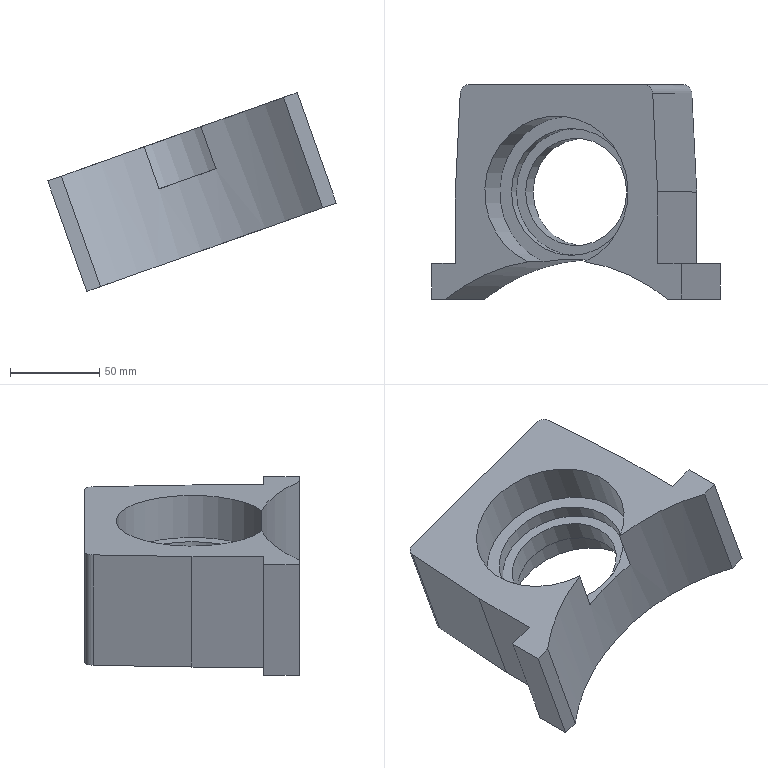Part | STEP file | SLIDE1-2_id582_x_t | 1 solid | 24 faces | box 161.375 x 120 x 111.146 mm | volume 535802 mm3 | plane 17 | cylinder 7 | commonest cylinder face diameters 10 x2 60 x1 71 x1 78 x1 85 x1 217 x1
STEP:
#1=CARTESIAN_POINT('',(-4.502,0.,-133.439));
#2=VERTEX_POINT('',#1);
#3=CARTESIAN_POINT('',(23.777,0.,-123.425));
#4=DIRECTION('',(-0.3338,0.,0.9426));
#5=DIRECTION('',(-0.9426,0.,-0.3338));
#6=AXIS2_PLACEMENT_3D('',#3,#4,#5);
#7=CIRCLE('',#6,30.);
#8=EDGE_CURVE('',#2,#2,#7,.T.);
#9=ORIENTED_EDGE('',*,*,#8,.F.);
#10=EDGE_LOOP('',(#9));
#11=FACE_BOUND('',#10,.T.);
#12=CARTESIAN_POINT('',(-8.675,0.,-121.656));
#13=VERTEX_POINT('',#12);
#14=CARTESIAN_POINT('',(19.605,0.,-111.642));
#15=DIRECTION('',(-0.3338,0.,0.9426));
#16=DIRECTION('',(-0.9426,0.,-0.3338));
#17=AXIS2_PLACEMENT_3D('',#14,#15,#16);
#18=CIRCLE('',#17,30.);
#19=EDGE_CURVE('',#13,#13,#18,.T.);
#20=ORIENTED_EDGE('',*,*,#19,.T.);
#21=EDGE_LOOP('',(#20));
#22=FACE_BOUND('',#21,.T.);
#23=CARTESIAN_POINT('',(23.777,0.,-123.425));
#24=DIRECTION('',(0.3338,0.,-0.9426));
#25=DIRECTION('',(-0.9426,0.,-0.3338));
#26=AXIS2_PLACEMENT_3D('',#23,#24,#25);
#27=CYLINDRICAL_SURFACE('',#26,30.);
#28=ADVANCED_FACE('',(#11,#22),#27,.F.);
#29=ORIENTED_EDGE('',*,*,#8,.T.);
#30=EDGE_LOOP('',(#29));
#31=FACE_BOUND('',#30,.T.);
#32=CARTESIAN_POINT('',(7.559,-35.,-129.168));
#33=VERTEX_POINT('',#32);
#34=CARTESIAN_POINT('',(39.995,-35.,-117.682));
#35=VERTEX_POINT('',#34);
#36=CARTESIAN_POINT('',(7.559,-35.,-129.168));
#37=DIRECTION('',(0.9426,0.,0.3338));
#38=VECTOR('',#37,1.);
#39=LINE('',#36,#38);
#40=EDGE_CURVE('',#33,#35,#39,.T.);
#41=ORIENTED_EDGE('',*,*,#40,.F.);
#42=CARTESIAN_POINT('',(23.777,0.,-123.425));
#43=DIRECTION('',(0.3338,0.,-0.9426));
#44=DIRECTION('',(-0.9426,0.,-0.3338));
#45=AXIS2_PLACEMENT_3D('',#42,#43,#44);
#46=CIRCLE('',#45,39.);
#47=EDGE_CURVE('',#33,#35,#46,.T.);
#48=ORIENTED_EDGE('',*,*,#47,.T.);
#49=EDGE_LOOP('',(#41,#48));
#50=FACE_BOUND('',#49,.T.);
#51=CARTESIAN_POINT('',(-32.781,60.,-143.453));
#52=DIRECTION('',(0.3338,0.,-0.9426));
#53=DIRECTION('',(-0.9426,0.,-0.3338));
#54=AXIS2_PLACEMENT_3D('',#51,#52,#53);
#55=PLANE('',#54);
#56=ADVANCED_FACE('',(#31,#50),#55,.T.);
#57=ORIENTED_EDGE('',*,*,#19,.F.);
#58=EDGE_LOOP('',(#57));
#59=FACE_BOUND('',#58,.T.);
#60=CARTESIAN_POINT('',(-13.859,0.,-123.492));
#61=VERTEX_POINT('',#60);
#62=CARTESIAN_POINT('',(19.605,0.,-111.642));
#63=DIRECTION('',(-0.3338,0.,0.9426));
#64=DIRECTION('',(-0.9426,0.,-0.3338));
#65=AXIS2_PLACEMENT_3D('',#62,#63,#64);
#66=CIRCLE('',#65,35.5);
#67=EDGE_CURVE('',#61,#61,#66,.T.);
#68=ORIENTED_EDGE('',*,*,#67,.T.);
#69=EDGE_LOOP('',(#68));
#70=FACE_BOUND('',#69,.T.);
#71=CARTESIAN_POINT('',(-36.954,60.,-131.67));
#72=DIRECTION('',(0.3338,0.,-0.9426));
#73=DIRECTION('',(-0.9426,0.,-0.3338));
#74=AXIS2_PLACEMENT_3D('',#71,#72,#73);
#75=PLANE('',#74);
#76=ADVANCED_FACE('',(#59,#70),#75,.F.);
#77=CARTESIAN_POINT('',(14.236,-35.,-148.021));
#78=VERTEX_POINT('',#77);
#79=CARTESIAN_POINT('',(14.236,-35.,-148.021));
#80=DIRECTION('',(-0.3338,0.,0.9426));
#81=VECTOR('',#80,1.);
#82=LINE('',#79,#81);
#83=EDGE_CURVE('',#78,#33,#82,.T.);
#84=ORIENTED_EDGE('',*,*,#83,.T.);
#85=ORIENTED_EDGE('',*,*,#40,.T.);
#86=CARTESIAN_POINT('',(46.671,-35.,-136.535));
#87=VERTEX_POINT('',#86);
#88=CARTESIAN_POINT('',(46.671,-35.,-136.535));
#89=DIRECTION('',(0.3338,0.,-0.9426));
#90=VECTOR('',#89,1.);
#91=LINE('',#88,#90);
#92=EDGE_CURVE('',#35,#87,#91,.T.);
#93=ORIENTED_EDGE('',*,*,#92,.T.);
#94=CARTESIAN_POINT('',(48.162,-35.,-136.007));
#95=DIRECTION('',(0.9426,0.,0.3338));
#96=VECTOR('',#95,1.);
#97=LINE('',#94,#96);
#98=EDGE_CURVE('',#78,#87,#97,.T.);
#99=ORIENTED_EDGE('',*,*,#98,.F.);
#100=EDGE_LOOP('',(#84,#85,#93,#99));
#101=FACE_OUTER_BOUND('',#100,.T.);
#102=CARTESIAN_POINT('',(7.559,-35.,-129.168));
#103=DIRECTION('',(0.,1.,0.));
#104=DIRECTION('',(0.,0.,1.));
#105=AXIS2_PLACEMENT_3D('',#102,#103,#104);
#106=PLANE('',#105);
#107=ADVANCED_FACE('',(#101),#106,.T.);
#108=ORIENTED_EDGE('',*,*,#47,.F.);
#109=ORIENTED_EDGE('',*,*,#83,.F.);
#110=CARTESIAN_POINT('',(30.453,0.,-142.278));
#111=DIRECTION('',(-0.3338,0.,0.9426));
#112=DIRECTION('',(-0.9426,0.,-0.3338));
#113=AXIS2_PLACEMENT_3D('',#110,#111,#112);
#114=CIRCLE('',#113,39.);
#115=EDGE_CURVE('',#87,#78,#114,.T.);
#116=ORIENTED_EDGE('',*,*,#115,.F.);
#117=ORIENTED_EDGE('',*,*,#92,.F.);
#118=EDGE_LOOP('',(#108,#109,#116,#117));
#119=FACE_OUTER_BOUND('',#118,.T.);
#120=CARTESIAN_POINT('',(30.453,0.,-142.278));
#121=DIRECTION('',(0.3338,0.,-0.9426));
#122=DIRECTION('',(-0.9426,0.,-0.3338));
#123=AXIS2_PLACEMENT_3D('',#120,#121,#122);
#124=CYLINDRICAL_SURFACE('',#123,39.);
#125=ADVANCED_FACE('',(#119),#124,.F.);
#126=ORIENTED_EDGE('',*,*,#67,.F.);
#127=EDGE_LOOP('',(#126));
#128=FACE_BOUND('',#127,.T.);
#129=CARTESIAN_POINT('',(-16.53,0.,-115.951));
#130=VERTEX_POINT('',#129);
#131=CARTESIAN_POINT('',(16.934,0.,-104.101));
#132=DIRECTION('',(-0.3338,0.,0.9426));
#133=DIRECTION('',(-0.9426,0.,-0.3338));
#134=AXIS2_PLACEMENT_3D('',#131,#132,#133);
#135=CIRCLE('',#134,35.5);
#136=EDGE_CURVE('',#130,#130,#135,.T.);
#137=ORIENTED_EDGE('',*,*,#136,.T.);
#138=EDGE_LOOP('',(#137));
#139=FACE_BOUND('',#138,.T.);
#140=CARTESIAN_POINT('',(19.605,0.,-111.642));
#141=DIRECTION('',(0.3338,0.,-0.9426));
#142=DIRECTION('',(-0.9426,0.,-0.3338));
#143=AXIS2_PLACEMENT_3D('',#140,#141,#142);
#144=CYLINDRICAL_SURFACE('',#143,35.5);
#145=ADVANCED_FACE('',(#128,#139),#144,.F.);
#146=CARTESIAN_POINT('',(57.711,60.,-63.14));
#147=VERTEX_POINT('',#146);
#148=CARTESIAN_POINT('',(62.418,55.262,-61.473));
#149=VERTEX_POINT('',#148);
#150=CARTESIAN_POINT('',(57.711,55.,-63.14));
#151=DIRECTION('',(0.3338,0.,-0.9426));
#152=DIRECTION('',(-0.9426,0.,-0.3338));
#153=AXIS2_PLACEMENT_3D('',#150,#151,#152);
#154=CIRCLE('',#153,5.);
#155=EDGE_CURVE('',#147,#149,#154,.T.);
#156=ORIENTED_EDGE('',*,*,#155,.T.);
#157=CARTESIAN_POINT('',(84.282,55.262,-123.216));
#158=VERTEX_POINT('',#157);
#159=CARTESIAN_POINT('',(62.418,55.262,-61.473));
#160=DIRECTION('',(0.3338,0.,-0.9426));
#161=VECTOR('',#160,1.);
#162=LINE('',#159,#161);
#163=EDGE_CURVE('',#149,#158,#162,.T.);
#164=ORIENTED_EDGE('',*,*,#163,.T.);
#165=CARTESIAN_POINT('',(79.575,60.,-124.883));
#166=VERTEX_POINT('',#165);
#167=CARTESIAN_POINT('',(79.575,55.,-124.883));
#168=DIRECTION('',(0.3338,0.,-0.9426));
#169=DIRECTION('',(-0.9426,0.,-0.3338));
#170=AXIS2_PLACEMENT_3D('',#167,#168,#169);
#171=CIRCLE('',#170,5.);
#172=EDGE_CURVE('',#166,#158,#171,.T.);
#173=ORIENTED_EDGE('',*,*,#172,.F.);
#174=CARTESIAN_POINT('',(57.711,60.,-63.14));
#175=DIRECTION('',(0.3338,0.,-0.9426));
#176=VECTOR('',#175,1.);
#177=LINE('',#174,#176);
#178=EDGE_CURVE('',#147,#166,#177,.T.);
#179=ORIENTED_EDGE('',*,*,#178,.F.);
#180=EDGE_LOOP('',(#156,#164,#173,#179));
#181=FACE_OUTER_BOUND('',#180,.T.);
#182=CARTESIAN_POINT('',(57.595,55.,-62.813));
#183=DIRECTION('',(0.3338,0.,-0.9426));
#184=DIRECTION('',(-0.9426,0.,-0.3338));
#185=AXIS2_PLACEMENT_3D('',#182,#183,#184);
#186=CYLINDRICAL_SURFACE('',#185,5.);
#187=ADVANCED_FACE('',(#181),#186,.T.);
#188=CARTESIAN_POINT('',(87.012,0.,-122.249));
#189=VERTEX_POINT('',#188);
#190=CARTESIAN_POINT('',(65.148,0.,-60.506));
#191=VERTEX_POINT('',#190);
#192=CARTESIAN_POINT('',(65.148,0.,-60.506));
#193=DIRECTION('',(-0.3338,0.,0.9426));
#194=VECTOR('',#193,1.);
#195=LINE('',#192,#194);
#196=EDGE_CURVE('',#189,#191,#195,.T.);
#197=ORIENTED_EDGE('',*,*,#196,.F.);
#198=CARTESIAN_POINT('',(84.282,55.262,-123.216));
#199=DIRECTION('',(0.04933,-0.9986,0.01747));
#200=VECTOR('',#199,1.);
#201=LINE('',#198,#200);
#202=EDGE_CURVE('',#158,#189,#201,.T.);
#203=ORIENTED_EDGE('',*,*,#202,.F.);
#204=ORIENTED_EDGE('',*,*,#163,.F.);
#205=CARTESIAN_POINT('',(62.418,55.262,-61.473));
#206=DIRECTION('',(0.04933,-0.9986,0.01747));
#207=VECTOR('',#206,1.);
#208=LINE('',#205,#207);
#209=EDGE_CURVE('',#149,#191,#208,.T.);
#210=ORIENTED_EDGE('',*,*,#209,.T.);
#211=EDGE_LOOP('',(#197,#203,#204,#210));
#212=FACE_OUTER_BOUND('',#211,.T.);
#213=CARTESIAN_POINT('',(62.183,60.,-61.556));
#214=DIRECTION('',(-0.9413,-0.05234,-0.3333));
#215=DIRECTION('',(-0.3338,0.,0.9426));
#216=AXIS2_PLACEMENT_3D('',#213,#214,#215);
#217=PLANE('',#216);
#218=ADVANCED_FACE('',(#212),#217,.F.);
#219=CARTESIAN_POINT('',(87.012,-40.,-122.249));
#220=VERTEX_POINT('',#219);
#221=CARTESIAN_POINT('',(87.012,60.,-122.249));
#222=DIRECTION('',(0.,-1.,0.));
#223=VECTOR('',#222,1.);
#224=LINE('',#221,#223);
#225=EDGE_CURVE('',#189,#220,#224,.T.);
#226=ORIENTED_EDGE('',*,*,#225,.F.);
#227=ORIENTED_EDGE('',*,*,#196,.T.);
#228=CARTESIAN_POINT('',(65.148,-40.,-60.506));
#229=VERTEX_POINT('',#228);
#230=CARTESIAN_POINT('',(65.148,60.,-60.506));
#231=DIRECTION('',(0.,-1.,0.));
#232=VECTOR('',#231,1.);
#233=LINE('',#230,#232);
#234=EDGE_CURVE('',#191,#229,#233,.T.);
#235=ORIENTED_EDGE('',*,*,#234,.T.);
#236=CARTESIAN_POINT('',(87.012,-40.,-122.249));
#237=DIRECTION('',(-0.3338,0.,0.9426));
#238=VECTOR('',#237,1.);
#239=LINE('',#236,#238);
#240=EDGE_CURVE('',#220,#229,#239,.T.);
#241=ORIENTED_EDGE('',*,*,#240,.F.);
#242=EDGE_LOOP('',(#226,#227,#235,#241));
#243=FACE_OUTER_BOUND('',#242,.T.);
#244=CARTESIAN_POINT('',(65.148,60.,-60.506));
#245=DIRECTION('',(0.9426,0.,0.3338));
#246=DIRECTION('',(0.3338,0.,-0.9426));
#247=AXIS2_PLACEMENT_3D('',#244,#245,#246);
#248=PLANE('',#247);
#249=ADVANCED_FACE('',(#243),#248,.T.);
#250=ORIENTED_EDGE('',*,*,#240,.T.);
#251=CARTESIAN_POINT('',(78.345,-40.,-55.833));
#252=VERTEX_POINT('',#251);
#253=CARTESIAN_POINT('',(26.298,-40.,-74.264));
#254=DIRECTION('',(0.9426,0.,0.3338));
#255=VECTOR('',#254,1.);
#256=LINE('',#253,#255);
#257=EDGE_CURVE('',#229,#252,#256,.T.);
#258=ORIENTED_EDGE('',*,*,#257,.T.);
#259=CARTESIAN_POINT('',(100.209,-40.,-117.576));
#260=VERTEX_POINT('',#259);
#261=CARTESIAN_POINT('',(78.345,-40.,-55.833));
#262=DIRECTION('',(-0.3338,0.,0.9426));
#263=VECTOR('',#262,1.);
#264=LINE('',#261,#263);
#265=EDGE_CURVE('',#260,#252,#264,.T.);
#266=ORIENTED_EDGE('',*,*,#265,.F.);
#267=CARTESIAN_POINT('',(48.162,-40.,-136.007));
#268=DIRECTION('',(0.9426,0.,0.3338));
#269=VECTOR('',#268,1.);
#270=LINE('',#267,#269);
#271=EDGE_CURVE('',#220,#260,#270,.T.);
#272=ORIENTED_EDGE('',*,*,#271,.F.);
#273=EDGE_LOOP('',(#250,#258,#266,#272));
#274=FACE_OUTER_BOUND('',#273,.T.);
#275=CARTESIAN_POINT('',(65.148,-40.,-60.506));
#276=DIRECTION('',(0.,1.,0.));
#277=DIRECTION('',(0.,0.,1.));
#278=AXIS2_PLACEMENT_3D('',#275,#276,#277);
#279=PLANE('',#278);
#280=ADVANCED_FACE('',(#274),#279,.T.);
#281=ORIENTED_EDGE('',*,*,#265,.T.);
#282=CARTESIAN_POINT('',(78.345,-60.,-55.833));
#283=VERTEX_POINT('',#282);
#284=CARTESIAN_POINT('',(78.345,60.,-55.833));
#285=DIRECTION('',(0.,-1.,0.));
#286=VECTOR('',#285,1.);
#287=LINE('',#284,#286);
#288=EDGE_CURVE('',#252,#283,#287,.T.);
#289=ORIENTED_EDGE('',*,*,#288,.T.);
#290=CARTESIAN_POINT('',(100.209,-60.,-117.576));
#291=VERTEX_POINT('',#290);
#292=CARTESIAN_POINT('',(100.209,-60.,-117.576));
#293=DIRECTION('',(-0.3338,0.,0.9426));
#294=VECTOR('',#293,1.);
#295=LINE('',#292,#294);
#296=EDGE_CURVE('',#291,#283,#295,.T.);
#297=ORIENTED_EDGE('',*,*,#296,.F.);
#298=CARTESIAN_POINT('',(100.209,60.,-117.576));
#299=DIRECTION('',(0.,-1.,0.));
#300=VECTOR('',#299,1.);
#301=LINE('',#298,#300);
#302=EDGE_CURVE('',#260,#291,#301,.T.);
#303=ORIENTED_EDGE('',*,*,#302,.F.);
#304=EDGE_LOOP('',(#281,#289,#297,#303));
#305=FACE_OUTER_BOUND('',#304,.T.);
#306=CARTESIAN_POINT('',(78.345,-50.,-55.833));
#307=DIRECTION('',(0.9426,0.,0.3338));
#308=DIRECTION('',(0.3338,0.,-0.9426));
#309=AXIS2_PLACEMENT_3D('',#306,#307,#308);
#310=PLANE('',#309);
#311=ADVANCED_FACE('',(#305),#310,.T.);
#312=CARTESIAN_POINT('',(-61.166,-60.,-105.236));
#313=VERTEX_POINT('',#312);
#314=CARTESIAN_POINT('',(-39.302,-60.,-166.979));
#315=VERTEX_POINT('',#314);
#316=CARTESIAN_POINT('',(-61.166,-60.,-105.236));
#317=DIRECTION('',(0.3338,0.,-0.9426));
#318=VECTOR('',#317,1.);
#319=LINE('',#316,#318);
#320=EDGE_CURVE('',#313,#315,#319,.T.);
#321=ORIENTED_EDGE('',*,*,#320,.F.);
#322=CARTESIAN_POINT('',(-61.166,-40.,-105.236));
#323=VERTEX_POINT('',#322);
#324=CARTESIAN_POINT('',(-61.166,60.,-105.236));
#325=DIRECTION('',(0.,1.,0.));
#326=VECTOR('',#325,1.);
#327=LINE('',#324,#326);
#328=EDGE_CURVE('',#313,#323,#327,.T.);
#329=ORIENTED_EDGE('',*,*,#328,.T.);
#330=CARTESIAN_POINT('',(-39.302,-40.,-166.979));
#331=VERTEX_POINT('',#330);
#332=CARTESIAN_POINT('',(-39.302,-40.,-166.979));
#333=DIRECTION('',(-0.3338,0.,0.9426));
#334=VECTOR('',#333,1.);
#335=LINE('',#332,#334);
#336=EDGE_CURVE('',#331,#323,#335,.T.);
#337=ORIENTED_EDGE('',*,*,#336,.F.);
#338=CARTESIAN_POINT('',(-39.302,60.,-166.979));
#339=DIRECTION('',(0.,1.,0.));
#340=VECTOR('',#339,1.);
#341=LINE('',#338,#340);
#342=EDGE_CURVE('',#315,#331,#341,.T.);
#343=ORIENTED_EDGE('',*,*,#342,.F.);
#344=EDGE_LOOP('',(#321,#329,#337,#343));
#345=FACE_OUTER_BOUND('',#344,.T.);
#346=CARTESIAN_POINT('',(-61.166,-60.,-105.236));
#347=DIRECTION('',(-0.9426,0.,-0.3338));
#348=DIRECTION('',(-0.3338,0.,0.9426));
#349=AXIS2_PLACEMENT_3D('',#346,#347,#348);
#350=PLANE('',#349);
#351=ADVANCED_FACE('',(#345),#350,.T.);
#352=ORIENTED_EDGE('',*,*,#336,.T.);
#353=CARTESIAN_POINT('',(-47.969,-40.,-100.563));
#354=VERTEX_POINT('',#353);
#355=CARTESIAN_POINT('',(26.298,-40.,-74.264));
#356=DIRECTION('',(0.9426,0.,0.3338));
#357=VECTOR('',#356,1.);
#358=LINE('',#355,#357);
#359=EDGE_CURVE('',#323,#354,#358,.T.);
#360=ORIENTED_EDGE('',*,*,#359,.T.);
#361=CARTESIAN_POINT('',(-26.105,-40.,-162.306));
#362=VERTEX_POINT('',#361);
#363=CARTESIAN_POINT('',(-47.969,-40.,-100.563));
#364=DIRECTION('',(-0.3338,0.,0.9426));
#365=VECTOR('',#364,1.);
#366=LINE('',#363,#365);
#367=EDGE_CURVE('',#362,#354,#366,.T.);
#368=ORIENTED_EDGE('',*,*,#367,.F.);
#369=CARTESIAN_POINT('',(48.162,-40.,-136.007));
#370=DIRECTION('',(0.9426,0.,0.3338));
#371=VECTOR('',#370,1.);
#372=LINE('',#369,#371);
#373=EDGE_CURVE('',#331,#362,#372,.T.);
#374=ORIENTED_EDGE('',*,*,#373,.F.);
#375=EDGE_LOOP('',(#352,#360,#368,#374));
#376=FACE_OUTER_BOUND('',#375,.T.);
#377=CARTESIAN_POINT('',(-55.511,-40.,-103.234));
#378=DIRECTION('',(0.,1.,0.));
#379=DIRECTION('',(0.,0.,1.));
#380=AXIS2_PLACEMENT_3D('',#377,#378,#379);
#381=PLANE('',#380);
#382=ADVANCED_FACE('',(#376),#381,.T.);
#383=CARTESIAN_POINT('',(-47.969,0.,-100.563));
#384=VERTEX_POINT('',#383);
#385=CARTESIAN_POINT('',(-47.969,60.,-100.563));
#386=DIRECTION('',(0.,1.,0.));
#387=VECTOR('',#386,1.);
#388=LINE('',#385,#387);
#389=EDGE_CURVE('',#354,#384,#388,.T.);
#390=ORIENTED_EDGE('',*,*,#389,.T.);
#391=CARTESIAN_POINT('',(-26.105,0.,-162.306));
#392=VERTEX_POINT('',#391);
#393=CARTESIAN_POINT('',(-47.969,0.,-100.563));
#394=DIRECTION('',(0.3338,0.,-0.9426));
#395=VECTOR('',#394,1.);
#396=LINE('',#393,#395);
#397=EDGE_CURVE('',#384,#392,#396,.T.);
#398=ORIENTED_EDGE('',*,*,#397,.T.);
#399=CARTESIAN_POINT('',(-26.105,60.,-162.306));
#400=DIRECTION('',(0.,1.,0.));
#401=VECTOR('',#400,1.);
#402=LINE('',#399,#401);
#403=EDGE_CURVE('',#362,#392,#402,.T.);
#404=ORIENTED_EDGE('',*,*,#403,.F.);
#405=ORIENTED_EDGE('',*,*,#367,.T.);
#406=EDGE_LOOP('',(#390,#398,#404,#405));
#407=FACE_OUTER_BOUND('',#406,.T.);
#408=CARTESIAN_POINT('',(-47.969,-50.,-100.563));
#409=DIRECTION('',(-0.9426,0.,-0.3338));
#410=DIRECTION('',(-0.3338,0.,0.9426));
#411=AXIS2_PLACEMENT_3D('',#408,#409,#410);
#412=PLANE('',#411);
#413=ADVANCED_FACE('',(#407),#412,.T.);
#414=ORIENTED_EDGE('',*,*,#397,.F.);
#415=CARTESIAN_POINT('',(-45.239,55.262,-99.596));
#416=VERTEX_POINT('',#415);
#417=CARTESIAN_POINT('',(-47.969,0.,-100.563));
#418=DIRECTION('',(0.04933,0.9986,0.01747));
#419=VECTOR('',#418,1.);
#420=LINE('',#417,#419);
#421=EDGE_CURVE('',#384,#416,#420,.T.);
#422=ORIENTED_EDGE('',*,*,#421,.T.);
#423=CARTESIAN_POINT('',(-23.375,55.262,-161.339));
#424=VERTEX_POINT('',#423);
#425=CARTESIAN_POINT('',(-23.273,55.262,-161.629));
#426=DIRECTION('',(-0.3338,0.,0.9426));
#427=VECTOR('',#426,1.);
#428=LINE('',#425,#427);
#429=EDGE_CURVE('',#424,#416,#428,.T.);
#430=ORIENTED_EDGE('',*,*,#429,.F.);
#431=CARTESIAN_POINT('',(-26.105,0.,-162.306));
#432=DIRECTION('',(0.04933,0.9986,0.01747));
#433=VECTOR('',#432,1.);
#434=LINE('',#431,#433);
#435=EDGE_CURVE('',#392,#424,#434,.T.);
#436=ORIENTED_EDGE('',*,*,#435,.F.);
#437=EDGE_LOOP('',(#414,#422,#430,#436));
#438=FACE_OUTER_BOUND('',#437,.T.);
#439=CARTESIAN_POINT('',(-47.969,0.,-100.563));
#440=DIRECTION('',(0.9413,-0.05234,0.3333));
#441=DIRECTION('',(0.3338,0.,-0.9426));
#442=AXIS2_PLACEMENT_3D('',#439,#440,#441);
#443=PLANE('',#442);
#444=ADVANCED_FACE('',(#438),#443,.F.);
#445=CARTESIAN_POINT('',(-18.668,60.,-159.673));
#446=VERTEX_POINT('',#445);
#447=CARTESIAN_POINT('',(-18.668,55.,-159.673));
#448=DIRECTION('',(0.3338,0.,-0.9426));
#449=DIRECTION('',(0.9426,0.,0.3338));
#450=AXIS2_PLACEMENT_3D('',#447,#448,#449);
#451=CIRCLE('',#450,5.);
#452=EDGE_CURVE('',#424,#446,#451,.T.);
#453=ORIENTED_EDGE('',*,*,#452,.F.);
#454=ORIENTED_EDGE('',*,*,#429,.T.);
#455=CARTESIAN_POINT('',(-40.533,60.,-97.93));
#456=VERTEX_POINT('',#455);
#457=CARTESIAN_POINT('',(-40.533,55.,-97.93));
#458=DIRECTION('',(0.3338,0.,-0.9426));
#459=DIRECTION('',(0.9426,0.,0.3338));
#460=AXIS2_PLACEMENT_3D('',#457,#458,#459);
#461=CIRCLE('',#460,5.);
#462=EDGE_CURVE('',#416,#456,#461,.T.);
#463=ORIENTED_EDGE('',*,*,#462,.T.);
#464=CARTESIAN_POINT('',(-18.668,60.,-159.673));
#465=DIRECTION('',(-0.3338,0.,0.9426));
#466=VECTOR('',#465,1.);
#467=LINE('',#464,#466);
#468=EDGE_CURVE('',#446,#456,#467,.T.);
#469=ORIENTED_EDGE('',*,*,#468,.F.);
#470=EDGE_LOOP('',(#453,#454,#463,#469));
#471=FACE_OUTER_BOUND('',#470,.T.);
#472=CARTESIAN_POINT('',(-18.566,55.,-159.962));
#473=DIRECTION('',(-0.3338,0.,0.9426));
#474=DIRECTION('',(0.9426,0.,0.3338));
#475=AXIS2_PLACEMENT_3D('',#472,#473,#474);
#476=CYLINDRICAL_SURFACE('',#475,5.);
#477=ADVANCED_FACE('',(#471),#476,.T.);
#478=CARTESIAN_POINT('',(26.298,60.,-74.264));
#479=DIRECTION('',(0.9426,0.,0.3338));
#480=VECTOR('',#479,1.);
#481=LINE('',#478,#480);
#482=EDGE_CURVE('',#456,#147,#481,.T.);
#483=ORIENTED_EDGE('',*,*,#482,.T.);
#484=ORIENTED_EDGE('',*,*,#178,.T.);
#485=CARTESIAN_POINT('',(48.162,60.,-136.007));
#486=DIRECTION('',(0.9426,0.,0.3338));
#487=VECTOR('',#486,1.);
#488=LINE('',#485,#487);
#489=EDGE_CURVE('',#446,#166,#488,.T.);
#490=ORIENTED_EDGE('',*,*,#489,.F.);
#491=ORIENTED_EDGE('',*,*,#468,.T.);
#492=EDGE_LOOP('',(#483,#484,#490,#491));
#493=FACE_OUTER_BOUND('',#492,.T.);
#494=CARTESIAN_POINT('',(-47.969,60.,-100.563));
#495=DIRECTION('',(0.,1.,0.));
#496=DIRECTION('',(0.,0.,1.));
#497=AXIS2_PLACEMENT_3D('',#494,#495,#496);
#498=PLANE('',#497);
#499=ADVANCED_FACE('',(#493),#498,.T.);
#500=CARTESIAN_POINT('',(70.702,-60.,-58.539));
#501=VERTEX_POINT('',#500);
#502=CARTESIAN_POINT('',(26.298,-60.,-74.264));
#503=DIRECTION('',(-0.9426,0.,-0.3338));
#504=VECTOR('',#503,1.);
#505=LINE('',#502,#504);
#506=EDGE_CURVE('',#283,#501,#505,.T.);
#507=ORIENTED_EDGE('',*,*,#506,.T.);
#508=CARTESIAN_POINT('',(92.566,-60.,-120.282));
#509=VERTEX_POINT('',#508);
#510=CARTESIAN_POINT('',(70.702,-60.,-58.539));
#511=DIRECTION('',(0.3338,0.,-0.9426));
#512=VECTOR('',#511,1.);
#513=LINE('',#510,#512);
#514=EDGE_CURVE('',#501,#509,#513,.T.);
#515=ORIENTED_EDGE('',*,*,#514,.T.);
#516=CARTESIAN_POINT('',(48.162,-60.,-136.007));
#517=DIRECTION('',(-0.9426,0.,-0.3338));
#518=VECTOR('',#517,1.);
#519=LINE('',#516,#518);
#520=EDGE_CURVE('',#291,#509,#519,.T.);
#521=ORIENTED_EDGE('',*,*,#520,.F.);
#522=ORIENTED_EDGE('',*,*,#296,.T.);
#523=EDGE_LOOP('',(#507,#515,#521,#522));
#524=FACE_OUTER_BOUND('',#523,.T.);
#525=CARTESIAN_POINT('',(72.689,-60.,-57.836));
#526=DIRECTION('',(0.,-1.,0.));
#527=DIRECTION('',(0.,0.,-1.));
#528=AXIS2_PLACEMENT_3D('',#525,#526,#527);
#529=PLANE('',#528);
#530=ADVANCED_FACE('',(#524),#529,.T.);
#531=ORIENTED_EDGE('',*,*,#98,.T.);
#532=ORIENTED_EDGE('',*,*,#115,.T.);
#533=EDGE_LOOP('',(#531,#532));
#534=FACE_BOUND('',#533,.T.);
#535=ORIENTED_EDGE('',*,*,#489,.T.);
#536=ORIENTED_EDGE('',*,*,#172,.T.);
#537=ORIENTED_EDGE('',*,*,#202,.T.);
#538=ORIENTED_EDGE('',*,*,#225,.T.);
#539=ORIENTED_EDGE('',*,*,#271,.T.);
#540=ORIENTED_EDGE('',*,*,#302,.T.);
#541=ORIENTED_EDGE('',*,*,#520,.T.);
#542=CARTESIAN_POINT('',(-31.66,-60.,-164.273));
#543=VERTEX_POINT('',#542);
#544=CARTESIAN_POINT('',(30.453,-146.2,-142.278));
#545=DIRECTION('',(-0.3338,0.,0.9426));
#546=DIRECTION('',(0.9426,0.,0.3338));
#547=AXIS2_PLACEMENT_3D('',#544,#545,#546);
#548=CIRCLE('',#547,108.5);
#549=EDGE_CURVE('',#509,#543,#548,.T.);
#550=ORIENTED_EDGE('',*,*,#549,.T.);
#551=CARTESIAN_POINT('',(-39.302,-60.,-166.979));
#552=DIRECTION('',(0.9426,0.,0.3338));
#553=VECTOR('',#552,1.);
#554=LINE('',#551,#553);
#555=EDGE_CURVE('',#315,#543,#554,.T.);
#556=ORIENTED_EDGE('',*,*,#555,.F.);
#557=ORIENTED_EDGE('',*,*,#342,.T.);
#558=ORIENTED_EDGE('',*,*,#373,.T.);
#559=ORIENTED_EDGE('',*,*,#403,.T.);
#560=ORIENTED_EDGE('',*,*,#435,.T.);
#561=ORIENTED_EDGE('',*,*,#452,.T.);
#562=EDGE_LOOP('',(#535,#536,#537,#538,#539,#540,#541,#550,#556,#557,#558,#559,#560,#561));
#563=FACE_BOUND('',#562,.T.);
#564=CARTESIAN_POINT('',(48.162,60.,-136.007));
#565=DIRECTION('',(0.3338,0.,-0.9426));
#566=DIRECTION('',(-0.9426,0.,-0.3338));
#567=AXIS2_PLACEMENT_3D('',#564,#565,#566);
#568=PLANE('',#567);
#569=ADVANCED_FACE('',(#534,#563),#568,.T.);
#570=ORIENTED_EDGE('',*,*,#555,.T.);
#571=CARTESIAN_POINT('',(-53.524,-60.,-102.53));
#572=VERTEX_POINT('',#571);
#573=CARTESIAN_POINT('',(-53.524,-60.,-102.53));
#574=DIRECTION('',(-0.3338,0.,0.9426));
#575=VECTOR('',#574,1.);
#576=LINE('',#573,#575);
#577=EDGE_CURVE('',#543,#572,#576,.T.);
#578=ORIENTED_EDGE('',*,*,#577,.T.);
#579=CARTESIAN_POINT('',(26.298,-60.,-74.264));
#580=DIRECTION('',(-0.9426,0.,-0.3338));
#581=VECTOR('',#580,1.);
#582=LINE('',#579,#581);
#583=EDGE_CURVE('',#572,#313,#582,.T.);
#584=ORIENTED_EDGE('',*,*,#583,.T.);
#585=ORIENTED_EDGE('',*,*,#320,.T.);
#586=EDGE_LOOP('',(#570,#578,#584,#585));
#587=FACE_OUTER_BOUND('',#586,.T.);
#588=CARTESIAN_POINT('',(72.689,-60.,-57.836));
#589=DIRECTION('',(0.,-1.,0.));
#590=DIRECTION('',(0.,0.,-1.));
#591=AXIS2_PLACEMENT_3D('',#588,#589,#590);
#592=PLANE('',#591);
#593=ADVANCED_FACE('',(#587),#592,.T.);
#594=ORIENTED_EDGE('',*,*,#136,.F.);
#595=EDGE_LOOP('',(#594));
#596=FACE_BOUND('',#595,.T.);
#597=CARTESIAN_POINT('',(1.05,-39.017,-109.726));
#598=VERTEX_POINT('',#597);
#599=CARTESIAN_POINT('',(32.819,-39.017,-98.476));
#600=VERTEX_POINT('',#599);
#601=CARTESIAN_POINT('',(16.934,-146.2,-104.101));
#602=DIRECTION('',(0.3338,0.,-0.9426));
#603=DIRECTION('',(0.9426,0.,0.3338));
#604=AXIS2_PLACEMENT_3D('',#601,#602,#603);
#605=CIRCLE('',#604,108.5);
#606=EDGE_CURVE('',#598,#600,#605,.T.);
#607=ORIENTED_EDGE('',*,*,#606,.T.);
#608=CARTESIAN_POINT('',(16.934,0.,-104.101));
#609=DIRECTION('',(-0.3338,0.,0.9426));
#610=DIRECTION('',(-0.9426,0.,-0.3338));
#611=AXIS2_PLACEMENT_3D('',#608,#609,#610);
#612=CIRCLE('',#611,42.5);
#613=EDGE_CURVE('',#600,#598,#612,.T.);
#614=ORIENTED_EDGE('',*,*,#613,.T.);
#615=EDGE_LOOP('',(#607,#614));
#616=FACE_BOUND('',#615,.T.);
#617=CARTESIAN_POINT('',(-39.624,60.,-124.129));
#618=DIRECTION('',(0.3338,0.,-0.9426));
#619=DIRECTION('',(-0.9426,0.,-0.3338));
#620=AXIS2_PLACEMENT_3D('',#617,#618,#619);
#621=PLANE('',#620);
#622=ADVANCED_FACE('',(#596,#616),#621,.F.);
#623=CARTESIAN_POINT('',(24.474,-39.017,-74.91));
#624=VERTEX_POINT('',#623);
#625=CARTESIAN_POINT('',(-7.295,-39.017,-86.16));
#626=VERTEX_POINT('',#625);
#627=CARTESIAN_POINT('',(8.589,0.,-80.535));
#628=DIRECTION('',(-0.3338,0.,0.9426));
#629=DIRECTION('',(-0.9426,0.,-0.3338));
#630=AXIS2_PLACEMENT_3D('',#627,#628,#629);
#631=CIRCLE('',#630,42.5);
#632=EDGE_CURVE('',#624,#626,#631,.T.);
#633=ORIENTED_EDGE('',*,*,#632,.T.);
#634=CARTESIAN_POINT('',(-7.295,-39.017,-86.16));
#635=DIRECTION('',(0.3338,0.,-0.9426));
#636=VECTOR('',#635,1.);
#637=LINE('',#634,#636);
#638=EDGE_CURVE('',#626,#598,#637,.T.);
#639=ORIENTED_EDGE('',*,*,#638,.T.);
#640=ORIENTED_EDGE('',*,*,#613,.F.);
#641=CARTESIAN_POINT('',(24.474,-39.017,-74.91));
#642=DIRECTION('',(-0.3338,0.,0.9426));
#643=VECTOR('',#642,1.);
#644=LINE('',#641,#643);
#645=EDGE_CURVE('',#600,#624,#644,.T.);
#646=ORIENTED_EDGE('',*,*,#645,.T.);
#647=EDGE_LOOP('',(#633,#639,#640,#646));
#648=FACE_OUTER_BOUND('',#647,.T.);
#649=CARTESIAN_POINT('',(16.934,0.,-104.101));
#650=DIRECTION('',(0.3338,0.,-0.9426));
#651=DIRECTION('',(-0.9426,0.,-0.3338));
#652=AXIS2_PLACEMENT_3D('',#649,#650,#651);
#653=CYLINDRICAL_SURFACE('',#652,42.5);
#654=ADVANCED_FACE('',(#648),#653,.F.);
#655=ORIENTED_EDGE('',*,*,#462,.F.);
#656=ORIENTED_EDGE('',*,*,#421,.F.);
#657=ORIENTED_EDGE('',*,*,#389,.F.);
#658=ORIENTED_EDGE('',*,*,#359,.F.);
#659=ORIENTED_EDGE('',*,*,#328,.F.);
#660=ORIENTED_EDGE('',*,*,#583,.F.);
#661=CARTESIAN_POINT('',(8.589,-146.2,-80.535));
#662=DIRECTION('',(0.3338,0.,-0.9426));
#663=DIRECTION('',(0.9426,0.,0.3338));
#664=AXIS2_PLACEMENT_3D('',#661,#662,#663);
#665=CIRCLE('',#664,108.5);
#666=EDGE_CURVE('',#572,#626,#665,.T.);
#667=ORIENTED_EDGE('',*,*,#666,.T.);
#668=ORIENTED_EDGE('',*,*,#632,.F.);
#669=CARTESIAN_POINT('',(8.589,-146.2,-80.535));
#670=DIRECTION('',(0.3338,0.,-0.9426));
#671=DIRECTION('',(0.9426,0.,0.3338));
#672=AXIS2_PLACEMENT_3D('',#669,#670,#671);
#673=CIRCLE('',#672,108.5);
#674=EDGE_CURVE('',#624,#501,#673,.T.);
#675=ORIENTED_EDGE('',*,*,#674,.T.);
#676=ORIENTED_EDGE('',*,*,#506,.F.);
#677=ORIENTED_EDGE('',*,*,#288,.F.);
#678=ORIENTED_EDGE('',*,*,#257,.F.);
#679=ORIENTED_EDGE('',*,*,#234,.F.);
#680=ORIENTED_EDGE('',*,*,#209,.F.);
#681=ORIENTED_EDGE('',*,*,#155,.F.);
#682=ORIENTED_EDGE('',*,*,#482,.F.);
#683=EDGE_LOOP('',(#655,#656,#657,#658,#659,#660,#667,#668,#675,#676,#677,#678,#679,#680,#681,#682));
#684=FACE_OUTER_BOUND('',#683,.T.);
#685=CARTESIAN_POINT('',(26.298,60.,-74.264));
#686=DIRECTION('',(0.3338,0.,-0.9426));
#687=DIRECTION('',(-0.9426,0.,-0.3338));
#688=AXIS2_PLACEMENT_3D('',#685,#686,#687);
#689=PLANE('',#688);
#690=ADVANCED_FACE('',(#684),#689,.F.);
#691=ORIENTED_EDGE('',*,*,#645,.F.);
#692=ORIENTED_EDGE('',*,*,#606,.F.);
#693=ORIENTED_EDGE('',*,*,#638,.F.);
#694=ORIENTED_EDGE('',*,*,#666,.F.);
#695=ORIENTED_EDGE('',*,*,#577,.F.);
#696=ORIENTED_EDGE('',*,*,#549,.F.);
#697=ORIENTED_EDGE('',*,*,#514,.F.);
#698=ORIENTED_EDGE('',*,*,#674,.F.);
#699=EDGE_LOOP('',(#691,#692,#693,#694,#695,#696,#697,#698));
#700=FACE_OUTER_BOUND('',#699,.T.);
#701=CARTESIAN_POINT('',(8.589,-146.2,-80.535));
#702=DIRECTION('',(-0.3338,0.,0.9426));
#703=DIRECTION('',(0.9426,0.,0.3338));
#704=AXIS2_PLACEMENT_3D('',#701,#702,#703);
#705=CYLINDRICAL_SURFACE('',#704,108.5);
#706=ADVANCED_FACE('',(#700),#705,.F.);
#707=CLOSED_SHELL('',(#28,#56,#76,#107,#125,#145,#187,#218,#249,#280,#311,#351,#382,#413,#444,#477,#499,#530,#569,#593,#622,#654,#690,#706));
#708=MANIFOLD_SOLID_BREP('',#707);
#709=(LENGTH_UNIT()NAMED_UNIT(*)SI_UNIT(.MILLI.,.METRE.));
#710=UNCERTAINTY_MEASURE_WITH_UNIT(LENGTH_MEASURE(0.00004123),#709,'','');
#711=(NAMED_UNIT(*)PLANE_ANGLE_UNIT()SI_UNIT($,.RADIAN.));
#712=PLANE_ANGLE_MEASURE_WITH_UNIT(PLANE_ANGLE_MEASURE(0.01745),#711);
#713=DIMENSIONAL_EXPONENTS(0.,0.,0.,0.,0.,0.,0.);
#714=(CONVERSION_BASED_UNIT('DEGREE',#712)NAMED_UNIT(#713)PLANE_ANGLE_UNIT());
#715=(NAMED_UNIT(*)SI_UNIT($,.STERADIAN.)SOLID_ANGLE_UNIT());
#716=(GEOMETRIC_REPRESENTATION_CONTEXT(3)GLOBAL_UNCERTAINTY_ASSIGNED_CONTEXT((#710))GLOBAL_UNIT_ASSIGNED_CONTEXT((#709,#714,#715))REPRESENTATION_CONTEXT('',''));
#717=ADVANCED_BREP_SHAPE_REPRESENTATION('',(#708),#716);